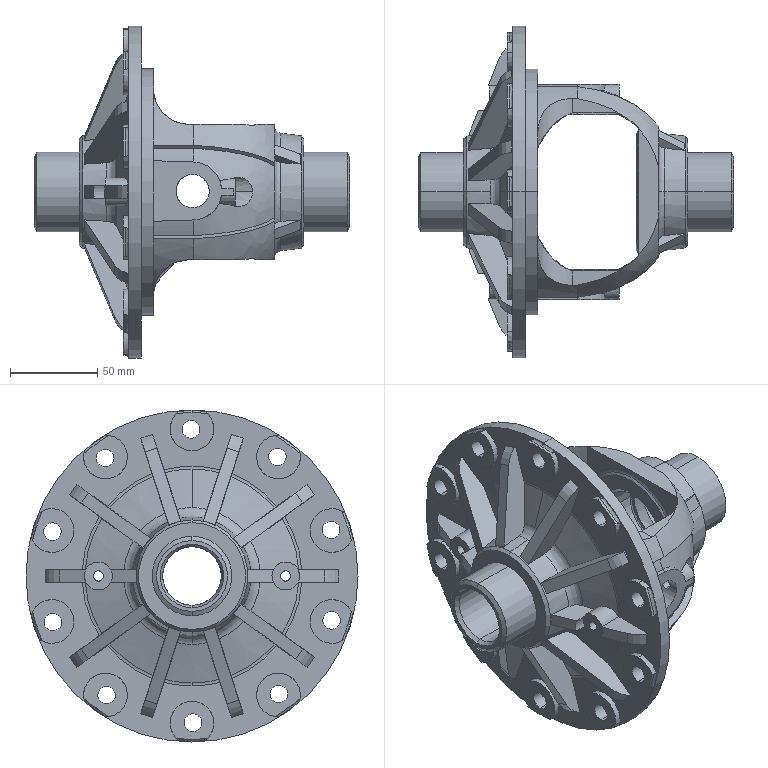Part | NX | features BREP 1 | 1 solid | 428 faces | box 180.42 x 190 x 190 mm | volume 596460 mm3 | plane 164 | cylinder 151 | torus 46 | spline 36 | cone 31 | commonest cylinder face diameters 25 x22 10 x20 5.9 x12 186.829 x11 16 x10 32 x10